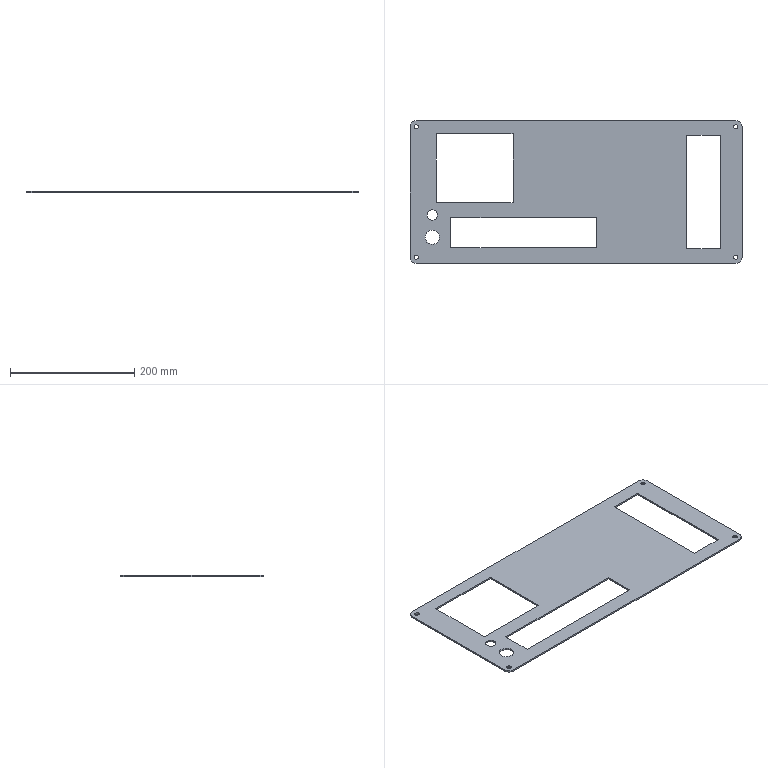Part | SolidWorks | features ICE 6, Extrusion 1, Fillet 1, LPattern 1 | 1 solid | 34 faces | box 535 x 230 x 2.5 mm | volume 217965 mm3 | plane 18 | cylinder 16 | commonest cylinder face diameters 7 x8 20 x4 16.5 x2 23 x2
STEP:
#1=CARTESIAN_POINT('',(27.75,-152.,0.));
#2=VERTEX_POINT('',#1);
#3=CARTESIAN_POINT('',(44.25,-152.,0.));
#4=VERTEX_POINT('',#3);
#5=CARTESIAN_POINT('',(36.,-152.,0.));
#6=DIRECTION('',(0.,0.,1.));
#7=DIRECTION('',(1.,0.,0.));
#8=AXIS2_PLACEMENT_3D('',#5,#6,#7);
#9=CIRCLE('',#8,8.25);
#10=EDGE_CURVE('',#2,#4,#9,.T.);
#11=ORIENTED_EDGE('',*,*,#10,.F.);
#12=CARTESIAN_POINT('',(27.75,-152.,2.5));
#13=VERTEX_POINT('',#12);
#14=CARTESIAN_POINT('',(27.75,-152.,0.));
#15=DIRECTION('',(0.,0.,1.));
#16=VECTOR('',#15,1000.);
#17=LINE('',#14,#16);
#18=EDGE_CURVE('',#2,#13,#17,.T.);
#19=ORIENTED_EDGE('',*,*,#18,.T.);
#20=CARTESIAN_POINT('',(44.25,-152.,2.5));
#21=VERTEX_POINT('',#20);
#22=CARTESIAN_POINT('',(36.,-152.,2.5));
#23=DIRECTION('',(0.,0.,1.));
#24=DIRECTION('',(1.,0.,0.));
#25=AXIS2_PLACEMENT_3D('',#22,#23,#24);
#26=CIRCLE('',#25,8.25);
#27=EDGE_CURVE('',#13,#21,#26,.T.);
#28=ORIENTED_EDGE('',*,*,#27,.T.);
#29=CARTESIAN_POINT('',(44.25,-152.,0.));
#30=DIRECTION('',(0.,0.,1.));
#31=VECTOR('',#30,1000.);
#32=LINE('',#29,#31);
#33=EDGE_CURVE('',#4,#21,#32,.T.);
#34=ORIENTED_EDGE('',*,*,#33,.F.);
#35=EDGE_LOOP('',(#11,#19,#28,#34));
#36=FACE_OUTER_BOUND('',#35,.T.);
#37=CARTESIAN_POINT('',(36.,-152.,0.));
#38=DIRECTION('',(0.,0.,1.));
#39=DIRECTION('',(1.,0.,0.));
#40=AXIS2_PLACEMENT_3D('',#37,#38,#39);
#41=CYLINDRICAL_SURFACE('',#40,8.25);
#42=ADVANCED_FACE('',(#36),#41,.F.);
#43=CARTESIAN_POINT('',(24.5,-188.,0.));
#44=VERTEX_POINT('',#43);
#45=CARTESIAN_POINT('',(47.5,-188.,0.));
#46=VERTEX_POINT('',#45);
#47=CARTESIAN_POINT('',(36.,-188.,0.));
#48=DIRECTION('',(0.,0.,1.));
#49=DIRECTION('',(1.,0.,0.));
#50=AXIS2_PLACEMENT_3D('',#47,#48,#49);
#51=CIRCLE('',#50,11.5);
#52=EDGE_CURVE('',#44,#46,#51,.T.);
#53=ORIENTED_EDGE('',*,*,#52,.F.);
#54=CARTESIAN_POINT('',(24.5,-188.,2.5));
#55=VERTEX_POINT('',#54);
#56=CARTESIAN_POINT('',(24.5,-188.,0.));
#57=DIRECTION('',(0.,0.,1.));
#58=VECTOR('',#57,1000.);
#59=LINE('',#56,#58);
#60=EDGE_CURVE('',#44,#55,#59,.T.);
#61=ORIENTED_EDGE('',*,*,#60,.T.);
#62=CARTESIAN_POINT('',(47.5,-188.,2.5));
#63=VERTEX_POINT('',#62);
#64=CARTESIAN_POINT('',(36.,-188.,2.5));
#65=DIRECTION('',(0.,0.,1.));
#66=DIRECTION('',(1.,0.,0.));
#67=AXIS2_PLACEMENT_3D('',#64,#65,#66);
#68=CIRCLE('',#67,11.5);
#69=EDGE_CURVE('',#55,#63,#68,.T.);
#70=ORIENTED_EDGE('',*,*,#69,.T.);
#71=CARTESIAN_POINT('',(47.5,-188.,0.));
#72=DIRECTION('',(0.,0.,1.));
#73=VECTOR('',#72,1000.);
#74=LINE('',#71,#73);
#75=EDGE_CURVE('',#46,#63,#74,.T.);
#76=ORIENTED_EDGE('',*,*,#75,.F.);
#77=EDGE_LOOP('',(#53,#61,#70,#76));
#78=FACE_OUTER_BOUND('',#77,.T.);
#79=CARTESIAN_POINT('',(36.,-188.,0.));
#80=DIRECTION('',(0.,0.,1.));
#81=DIRECTION('',(1.,0.,0.));
#82=AXIS2_PLACEMENT_3D('',#79,#80,#81);
#83=CYLINDRICAL_SURFACE('',#82,11.5);
#84=ADVANCED_FACE('',(#78),#83,.F.);
#85=CARTESIAN_POINT('',(521.5,-220.,0.));
#86=VERTEX_POINT('',#85);
#87=CARTESIAN_POINT('',(528.5,-220.,0.));
#88=VERTEX_POINT('',#87);
#89=CARTESIAN_POINT('',(525.,-220.,0.));
#90=DIRECTION('',(0.,0.,1.));
#91=DIRECTION('',(1.,0.,0.));
#92=AXIS2_PLACEMENT_3D('',#89,#90,#91);
#93=CIRCLE('',#92,3.5);
#94=EDGE_CURVE('',#86,#88,#93,.T.);
#95=ORIENTED_EDGE('',*,*,#94,.F.);
#96=CARTESIAN_POINT('',(521.5,-220.,2.5));
#97=VERTEX_POINT('',#96);
#98=CARTESIAN_POINT('',(521.5,-220.,0.));
#99=DIRECTION('',(0.,0.,1.));
#100=VECTOR('',#99,1000.);
#101=LINE('',#98,#100);
#102=EDGE_CURVE('',#86,#97,#101,.T.);
#103=ORIENTED_EDGE('',*,*,#102,.T.);
#104=CARTESIAN_POINT('',(528.5,-220.,2.5));
#105=VERTEX_POINT('',#104);
#106=CARTESIAN_POINT('',(525.,-220.,2.5));
#107=DIRECTION('',(0.,0.,1.));
#108=DIRECTION('',(1.,0.,0.));
#109=AXIS2_PLACEMENT_3D('',#106,#107,#108);
#110=CIRCLE('',#109,3.5);
#111=EDGE_CURVE('',#97,#105,#110,.T.);
#112=ORIENTED_EDGE('',*,*,#111,.T.);
#113=CARTESIAN_POINT('',(528.5,-220.,0.));
#114=DIRECTION('',(0.,0.,1.));
#115=VECTOR('',#114,1000.);
#116=LINE('',#113,#115);
#117=EDGE_CURVE('',#88,#105,#116,.T.);
#118=ORIENTED_EDGE('',*,*,#117,.F.);
#119=EDGE_LOOP('',(#95,#103,#112,#118));
#120=FACE_OUTER_BOUND('',#119,.T.);
#121=CARTESIAN_POINT('',(525.,-220.,0.));
#122=DIRECTION('',(0.,0.,1.));
#123=DIRECTION('',(1.,0.,0.));
#124=AXIS2_PLACEMENT_3D('',#121,#122,#123);
#125=CYLINDRICAL_SURFACE('',#124,3.5);
#126=ADVANCED_FACE('',(#120),#125,.F.);
#127=CARTESIAN_POINT('',(521.5,-10.,0.));
#128=VERTEX_POINT('',#127);
#129=CARTESIAN_POINT('',(528.5,-10.,0.));
#130=VERTEX_POINT('',#129);
#131=CARTESIAN_POINT('',(525.,-10.,0.));
#132=DIRECTION('',(0.,0.,1.));
#133=DIRECTION('',(1.,0.,0.));
#134=AXIS2_PLACEMENT_3D('',#131,#132,#133);
#135=CIRCLE('',#134,3.5);
#136=EDGE_CURVE('',#128,#130,#135,.T.);
#137=ORIENTED_EDGE('',*,*,#136,.F.);
#138=CARTESIAN_POINT('',(521.5,-10.,2.5));
#139=VERTEX_POINT('',#138);
#140=CARTESIAN_POINT('',(521.5,-10.,0.));
#141=DIRECTION('',(0.,0.,1.));
#142=VECTOR('',#141,1000.);
#143=LINE('',#140,#142);
#144=EDGE_CURVE('',#128,#139,#143,.T.);
#145=ORIENTED_EDGE('',*,*,#144,.T.);
#146=CARTESIAN_POINT('',(528.5,-10.,2.5));
#147=VERTEX_POINT('',#146);
#148=CARTESIAN_POINT('',(525.,-10.,2.5));
#149=DIRECTION('',(0.,0.,1.));
#150=DIRECTION('',(1.,0.,0.));
#151=AXIS2_PLACEMENT_3D('',#148,#149,#150);
#152=CIRCLE('',#151,3.5);
#153=EDGE_CURVE('',#139,#147,#152,.T.);
#154=ORIENTED_EDGE('',*,*,#153,.T.);
#155=CARTESIAN_POINT('',(528.5,-10.,0.));
#156=DIRECTION('',(0.,0.,1.));
#157=VECTOR('',#156,1000.);
#158=LINE('',#155,#157);
#159=EDGE_CURVE('',#130,#147,#158,.T.);
#160=ORIENTED_EDGE('',*,*,#159,.F.);
#161=EDGE_LOOP('',(#137,#145,#154,#160));
#162=FACE_OUTER_BOUND('',#161,.T.);
#163=CARTESIAN_POINT('',(525.,-10.,0.));
#164=DIRECTION('',(0.,0.,1.));
#165=DIRECTION('',(1.,0.,0.));
#166=AXIS2_PLACEMENT_3D('',#163,#164,#165);
#167=CYLINDRICAL_SURFACE('',#166,3.5);
#168=ADVANCED_FACE('',(#162),#167,.F.);
#169=CARTESIAN_POINT('',(6.5,-220.,0.));
#170=VERTEX_POINT('',#169);
#171=CARTESIAN_POINT('',(13.5,-220.,0.));
#172=VERTEX_POINT('',#171);
#173=CARTESIAN_POINT('',(10.,-220.,0.));
#174=DIRECTION('',(0.,0.,1.));
#175=DIRECTION('',(1.,0.,0.));
#176=AXIS2_PLACEMENT_3D('',#173,#174,#175);
#177=CIRCLE('',#176,3.5);
#178=EDGE_CURVE('',#170,#172,#177,.T.);
#179=ORIENTED_EDGE('',*,*,#178,.F.);
#180=CARTESIAN_POINT('',(6.5,-220.,2.5));
#181=VERTEX_POINT('',#180);
#182=CARTESIAN_POINT('',(6.5,-220.,0.));
#183=DIRECTION('',(0.,0.,1.));
#184=VECTOR('',#183,1000.);
#185=LINE('',#182,#184);
#186=EDGE_CURVE('',#170,#181,#185,.T.);
#187=ORIENTED_EDGE('',*,*,#186,.T.);
#188=CARTESIAN_POINT('',(13.5,-220.,2.5));
#189=VERTEX_POINT('',#188);
#190=CARTESIAN_POINT('',(10.,-220.,2.5));
#191=DIRECTION('',(0.,0.,1.));
#192=DIRECTION('',(1.,0.,0.));
#193=AXIS2_PLACEMENT_3D('',#190,#191,#192);
#194=CIRCLE('',#193,3.5);
#195=EDGE_CURVE('',#181,#189,#194,.T.);
#196=ORIENTED_EDGE('',*,*,#195,.T.);
#197=CARTESIAN_POINT('',(13.5,-220.,0.));
#198=DIRECTION('',(0.,0.,1.));
#199=VECTOR('',#198,1000.);
#200=LINE('',#197,#199);
#201=EDGE_CURVE('',#172,#189,#200,.T.);
#202=ORIENTED_EDGE('',*,*,#201,.F.);
#203=EDGE_LOOP('',(#179,#187,#196,#202));
#204=FACE_OUTER_BOUND('',#203,.T.);
#205=CARTESIAN_POINT('',(10.,-220.,0.));
#206=DIRECTION('',(0.,0.,1.));
#207=DIRECTION('',(1.,0.,0.));
#208=AXIS2_PLACEMENT_3D('',#205,#206,#207);
#209=CYLINDRICAL_SURFACE('',#208,3.5);
#210=ADVANCED_FACE('',(#204),#209,.F.);
#211=CARTESIAN_POINT('',(6.5,-10.,0.));
#212=VERTEX_POINT('',#211);
#213=CARTESIAN_POINT('',(13.5,-10.,0.));
#214=VERTEX_POINT('',#213);
#215=CARTESIAN_POINT('',(10.,-10.,0.));
#216=DIRECTION('',(0.,0.,1.));
#217=DIRECTION('',(1.,0.,0.));
#218=AXIS2_PLACEMENT_3D('',#215,#216,#217);
#219=CIRCLE('',#218,3.5);
#220=EDGE_CURVE('',#212,#214,#219,.T.);
#221=ORIENTED_EDGE('',*,*,#220,.F.);
#222=CARTESIAN_POINT('',(6.5,-10.,2.5));
#223=VERTEX_POINT('',#222);
#224=CARTESIAN_POINT('',(6.5,-10.,0.));
#225=DIRECTION('',(0.,0.,1.));
#226=VECTOR('',#225,1000.);
#227=LINE('',#224,#226);
#228=EDGE_CURVE('',#212,#223,#227,.T.);
#229=ORIENTED_EDGE('',*,*,#228,.T.);
#230=CARTESIAN_POINT('',(13.5,-10.,2.5));
#231=VERTEX_POINT('',#230);
#232=CARTESIAN_POINT('',(10.,-10.,2.5));
#233=DIRECTION('',(0.,0.,1.));
#234=DIRECTION('',(1.,0.,0.));
#235=AXIS2_PLACEMENT_3D('',#232,#233,#234);
#236=CIRCLE('',#235,3.5);
#237=EDGE_CURVE('',#223,#231,#236,.T.);
#238=ORIENTED_EDGE('',*,*,#237,.T.);
#239=CARTESIAN_POINT('',(13.5,-10.,0.));
#240=DIRECTION('',(0.,0.,1.));
#241=VECTOR('',#240,1000.);
#242=LINE('',#239,#241);
#243=EDGE_CURVE('',#214,#231,#242,.T.);
#244=ORIENTED_EDGE('',*,*,#243,.F.);
#245=EDGE_LOOP('',(#221,#229,#238,#244));
#246=FACE_OUTER_BOUND('',#245,.T.);
#247=CARTESIAN_POINT('',(10.,-10.,0.));
#248=DIRECTION('',(0.,0.,1.));
#249=DIRECTION('',(1.,0.,0.));
#250=AXIS2_PLACEMENT_3D('',#247,#248,#249);
#251=CYLINDRICAL_SURFACE('',#250,3.5);
#252=ADVANCED_FACE('',(#246),#251,.F.);
#253=CARTESIAN_POINT('',(0.,-10.,0.));
#254=VERTEX_POINT('',#253);
#255=CARTESIAN_POINT('',(0.,-220.,0.));
#256=VERTEX_POINT('',#255);
#257=CARTESIAN_POINT('',(0.,0.,0.));
#258=DIRECTION('',(0.,-1.,0.));
#259=VECTOR('',#258,1000.);
#260=LINE('',#257,#259);
#261=EDGE_CURVE('',#254,#256,#260,.T.);
#262=ORIENTED_EDGE('',*,*,#261,.T.);
#263=CARTESIAN_POINT('',(0.,-220.,2.5));
#264=VERTEX_POINT('',#263);
#265=CARTESIAN_POINT('',(0.,-220.,2.5));
#266=DIRECTION('',(0.,0.,1.));
#267=VECTOR('',#266,1000.);
#268=LINE('',#265,#267);
#269=EDGE_CURVE('',#256,#264,#268,.T.);
#270=ORIENTED_EDGE('',*,*,#269,.T.);
#271=CARTESIAN_POINT('',(0.,-10.,2.5));
#272=VERTEX_POINT('',#271);
#273=CARTESIAN_POINT('',(0.,0.,2.5));
#274=DIRECTION('',(0.,-1.,0.));
#275=VECTOR('',#274,1000.);
#276=LINE('',#273,#275);
#277=EDGE_CURVE('',#272,#264,#276,.T.);
#278=ORIENTED_EDGE('',*,*,#277,.F.);
#279=CARTESIAN_POINT('',(0.,-10.,2.5));
#280=DIRECTION('',(0.,0.,-1.));
#281=VECTOR('',#280,1000.);
#282=LINE('',#279,#281);
#283=EDGE_CURVE('',#272,#254,#282,.T.);
#284=ORIENTED_EDGE('',*,*,#283,.T.);
#285=EDGE_LOOP('',(#262,#270,#278,#284));
#286=FACE_OUTER_BOUND('',#285,.T.);
#287=CARTESIAN_POINT('',(0.,0.,2.5));
#288=DIRECTION('',(1.,0.,0.));
#289=DIRECTION('',(0.,1.,0.));
#290=AXIS2_PLACEMENT_3D('',#287,#288,#289);
#291=PLANE('',#290);
#292=ADVANCED_FACE('',(#286),#291,.F.);
#293=CARTESIAN_POINT('',(10.,-230.,2.5));
#294=VERTEX_POINT('',#293);
#295=CARTESIAN_POINT('',(525.,-230.,2.5));
#296=VERTEX_POINT('',#295);
#297=CARTESIAN_POINT('',(0.,-230.,2.5));
#298=DIRECTION('',(1.,0.,0.));
#299=VECTOR('',#298,1000.);
#300=LINE('',#297,#299);
#301=EDGE_CURVE('',#294,#296,#300,.T.);
#302=ORIENTED_EDGE('',*,*,#301,.F.);
#303=CARTESIAN_POINT('',(10.,-230.,0.));
#304=VERTEX_POINT('',#303);
#305=CARTESIAN_POINT('',(10.,-230.,2.5));
#306=DIRECTION('',(0.,0.,-1.));
#307=VECTOR('',#306,1000.);
#308=LINE('',#305,#307);
#309=EDGE_CURVE('',#294,#304,#308,.T.);
#310=ORIENTED_EDGE('',*,*,#309,.T.);
#311=CARTESIAN_POINT('',(525.,-230.,0.));
#312=VERTEX_POINT('',#311);
#313=CARTESIAN_POINT('',(0.,-230.,0.));
#314=DIRECTION('',(1.,0.,0.));
#315=VECTOR('',#314,1000.);
#316=LINE('',#313,#315);
#317=EDGE_CURVE('',#304,#312,#316,.T.);
#318=ORIENTED_EDGE('',*,*,#317,.T.);
#319=CARTESIAN_POINT('',(525.,-230.,2.5));
#320=DIRECTION('',(0.,0.,1.));
#321=VECTOR('',#320,1000.);
#322=LINE('',#319,#321);
#323=EDGE_CURVE('',#312,#296,#322,.T.);
#324=ORIENTED_EDGE('',*,*,#323,.T.);
#325=EDGE_LOOP('',(#302,#310,#318,#324));
#326=FACE_OUTER_BOUND('',#325,.T.);
#327=CARTESIAN_POINT('',(0.,-230.,2.5));
#328=DIRECTION('',(0.,1.,0.));
#329=DIRECTION('',(0.,0.,1.));
#330=AXIS2_PLACEMENT_3D('',#327,#328,#329);
#331=PLANE('',#330);
#332=ADVANCED_FACE('',(#326),#331,.F.);
#333=CARTESIAN_POINT('',(535.,-220.,2.5));
#334=VERTEX_POINT('',#333);
#335=CARTESIAN_POINT('',(535.,-10.,2.5));
#336=VERTEX_POINT('',#335);
#337=CARTESIAN_POINT('',(535.,0.,2.5));
#338=DIRECTION('',(0.,1.,0.));
#339=VECTOR('',#338,1000.);
#340=LINE('',#337,#339);
#341=EDGE_CURVE('',#334,#336,#340,.T.);
#342=ORIENTED_EDGE('',*,*,#341,.F.);
#343=CARTESIAN_POINT('',(535.,-220.,0.));
#344=VERTEX_POINT('',#343);
#345=CARTESIAN_POINT('',(535.,-220.,2.5));
#346=DIRECTION('',(0.,0.,-1.));
#347=VECTOR('',#346,1000.);
#348=LINE('',#345,#347);
#349=EDGE_CURVE('',#334,#344,#348,.T.);
#350=ORIENTED_EDGE('',*,*,#349,.T.);
#351=CARTESIAN_POINT('',(535.,-10.,0.));
#352=VERTEX_POINT('',#351);
#353=CARTESIAN_POINT('',(535.,0.,0.));
#354=DIRECTION('',(0.,1.,0.));
#355=VECTOR('',#354,1000.);
#356=LINE('',#353,#355);
#357=EDGE_CURVE('',#344,#352,#356,.T.);
#358=ORIENTED_EDGE('',*,*,#357,.T.);
#359=CARTESIAN_POINT('',(535.,-10.,2.5));
#360=DIRECTION('',(0.,0.,1.));
#361=VECTOR('',#360,1000.);
#362=LINE('',#359,#361);
#363=EDGE_CURVE('',#352,#336,#362,.T.);
#364=ORIENTED_EDGE('',*,*,#363,.T.);
#365=EDGE_LOOP('',(#342,#350,#358,#364));
#366=FACE_OUTER_BOUND('',#365,.T.);
#367=CARTESIAN_POINT('',(535.,0.,2.5));
#368=DIRECTION('',(-1.,0.,0.));
#369=DIRECTION('',(0.,0.,1.));
#370=AXIS2_PLACEMENT_3D('',#367,#368,#369);
#371=PLANE('',#370);
#372=ADVANCED_FACE('',(#366),#371,.F.);
#373=CARTESIAN_POINT('',(525.,0.,2.5));
#374=VERTEX_POINT('',#373);
#375=CARTESIAN_POINT('',(10.,0.,2.5));
#376=VERTEX_POINT('',#375);
#377=CARTESIAN_POINT('',(0.,0.,2.5));
#378=DIRECTION('',(-1.,0.,0.));
#379=VECTOR('',#378,1000.);
#380=LINE('',#377,#379);
#381=EDGE_CURVE('',#374,#376,#380,.T.);
#382=ORIENTED_EDGE('',*,*,#381,.F.);
#383=CARTESIAN_POINT('',(525.,0.,0.));
#384=VERTEX_POINT('',#383);
#385=CARTESIAN_POINT('',(525.,0.,2.5));
#386=DIRECTION('',(0.,0.,-1.));
#387=VECTOR('',#386,1000.);
#388=LINE('',#385,#387);
#389=EDGE_CURVE('',#374,#384,#388,.T.);
#390=ORIENTED_EDGE('',*,*,#389,.T.);
#391=CARTESIAN_POINT('',(10.,0.,0.));
#392=VERTEX_POINT('',#391);
#393=CARTESIAN_POINT('',(0.,0.,0.));
#394=DIRECTION('',(-1.,0.,0.));
#395=VECTOR('',#394,1000.);
#396=LINE('',#393,#395);
#397=EDGE_CURVE('',#384,#392,#396,.T.);
#398=ORIENTED_EDGE('',*,*,#397,.T.);
#399=CARTESIAN_POINT('',(10.,0.,2.5));
#400=DIRECTION('',(0.,0.,1.));
#401=VECTOR('',#400,1000.);
#402=LINE('',#399,#401);
#403=EDGE_CURVE('',#392,#376,#402,.T.);
#404=ORIENTED_EDGE('',*,*,#403,.T.);
#405=EDGE_LOOP('',(#382,#390,#398,#404));
#406=FACE_OUTER_BOUND('',#405,.T.);
#407=CARTESIAN_POINT('',(0.,0.,2.5));
#408=DIRECTION('',(0.,-1.,0.));
#409=DIRECTION('',(0.,0.,-1.));
#410=AXIS2_PLACEMENT_3D('',#407,#408,#409);
#411=PLANE('',#410);
#412=ADVANCED_FACE('',(#406),#411,.F.);
#413=CARTESIAN_POINT('',(446.,-23.5,2.5));
#414=VERTEX_POINT('',#413);
#415=CARTESIAN_POINT('',(446.,-206.5,2.5));
#416=VERTEX_POINT('',#415);
#417=CARTESIAN_POINT('',(446.,-23.5,2.5));
#418=DIRECTION('',(0.,-1.,0.));
#419=VECTOR('',#418,1000.);
#420=LINE('',#417,#419);
#421=EDGE_CURVE('',#414,#416,#420,.T.);
#422=ORIENTED_EDGE('',*,*,#421,.F.);
#423=CARTESIAN_POINT('',(500.,-23.5,2.5));
#424=VERTEX_POINT('',#423);
#425=CARTESIAN_POINT('',(446.,-23.5,2.5));
#426=DIRECTION('',(-1.,0.,0.));
#427=VECTOR('',#426,1000.);
#428=LINE('',#425,#427);
#429=EDGE_CURVE('',#424,#414,#428,.T.);
#430=ORIENTED_EDGE('',*,*,#429,.F.);
#431=CARTESIAN_POINT('',(500.,-206.5,2.5));
#432=VERTEX_POINT('',#431);
#433=CARTESIAN_POINT('',(500.,-23.5,2.5));
#434=DIRECTION('',(0.,1.,0.));
#435=VECTOR('',#434,1000.);
#436=LINE('',#433,#435);
#437=EDGE_CURVE('',#432,#424,#436,.T.);
#438=ORIENTED_EDGE('',*,*,#437,.F.);
#439=CARTESIAN_POINT('',(446.,-206.5,2.5));
#440=DIRECTION('',(1.,0.,0.));
#441=VECTOR('',#440,1000.);
#442=LINE('',#439,#441);
#443=EDGE_CURVE('',#416,#432,#442,.T.);
#444=ORIENTED_EDGE('',*,*,#443,.F.);
#445=EDGE_LOOP('',(#422,#430,#438,#444));
#446=FACE_BOUND('',#445,.T.);
#447=CARTESIAN_POINT('',(36.,-152.,2.5));
#448=DIRECTION('',(0.,0.,1.));
#449=DIRECTION('',(1.,0.,0.));
#450=AXIS2_PLACEMENT_3D('',#447,#448,#449);
#451=CIRCLE('',#450,8.25);
#452=EDGE_CURVE('',#21,#13,#451,.T.);
#453=ORIENTED_EDGE('',*,*,#452,.F.);
#454=ORIENTED_EDGE('',*,*,#27,.F.);
#455=EDGE_LOOP('',(#453,#454));
#456=FACE_BOUND('',#455,.T.);
#457=CARTESIAN_POINT('',(36.,-188.,2.5));
#458=DIRECTION('',(0.,0.,1.));
#459=DIRECTION('',(1.,0.,0.));
#460=AXIS2_PLACEMENT_3D('',#457,#458,#459);
#461=CIRCLE('',#460,11.5);
#462=EDGE_CURVE('',#63,#55,#461,.T.);
#463=ORIENTED_EDGE('',*,*,#462,.F.);
#464=ORIENTED_EDGE('',*,*,#69,.F.);
#465=EDGE_LOOP('',(#463,#464));
#466=FACE_BOUND('',#465,.T.);
#467=CARTESIAN_POINT('',(66.,-156.5,2.5));
#468=VERTEX_POINT('',#467);
#469=CARTESIAN_POINT('',(66.,-205.,2.5));
#470=VERTEX_POINT('',#469);
#471=CARTESIAN_POINT('',(66.,-156.5,2.5));
#472=DIRECTION('',(0.,-1.,0.));
#473=VECTOR('',#472,1000.);
#474=LINE('',#471,#473);
#475=EDGE_CURVE('',#468,#470,#474,.T.);
#476=ORIENTED_EDGE('',*,*,#475,.F.);
#477=CARTESIAN_POINT('',(300.,-156.5,2.5));
#478=VERTEX_POINT('',#477);
#479=CARTESIAN_POINT('',(66.,-156.5,2.5));
#480=DIRECTION('',(-1.,0.,0.));
#481=VECTOR('',#480,1000.);
#482=LINE('',#479,#481);
#483=EDGE_CURVE('',#478,#468,#482,.T.);
#484=ORIENTED_EDGE('',*,*,#483,.F.);
#485=CARTESIAN_POINT('',(300.,-205.,2.5));
#486=VERTEX_POINT('',#485);
#487=CARTESIAN_POINT('',(300.,-156.5,2.5));
#488=DIRECTION('',(0.,1.,0.));
#489=VECTOR('',#488,1000.);
#490=LINE('',#487,#489);
#491=EDGE_CURVE('',#486,#478,#490,.T.);
#492=ORIENTED_EDGE('',*,*,#491,.F.);
#493=CARTESIAN_POINT('',(66.,-205.,2.5));
#494=DIRECTION('',(1.,0.,0.));
#495=VECTOR('',#494,1000.);
#496=LINE('',#493,#495);
#497=EDGE_CURVE('',#470,#486,#496,.T.);
#498=ORIENTED_EDGE('',*,*,#497,.F.);
#499=EDGE_LOOP('',(#476,#484,#492,#498));
#500=FACE_BOUND('',#499,.T.);
#501=CARTESIAN_POINT('',(42.,-21.,2.5));
#502=VERTEX_POINT('',#501);
#503=CARTESIAN_POINT('',(42.,-132.,2.5));
#504=VERTEX_POINT('',#503);
#505=CARTESIAN_POINT('',(42.,-21.,2.5));
#506=DIRECTION('',(0.,-1.,0.));
#507=VECTOR('',#506,1000.);
#508=LINE('',#505,#507);
#509=EDGE_CURVE('',#502,#504,#508,.T.);
#510=ORIENTED_EDGE('',*,*,#509,.F.);
#511=CARTESIAN_POINT('',(166.,-21.,2.5));
#512=VERTEX_POINT('',#511);
#513=CARTESIAN_POINT('',(42.,-21.,2.5));
#514=DIRECTION('',(-1.,0.,0.));
#515=VECTOR('',#514,1000.);
#516=LINE('',#513,#515);
#517=EDGE_CURVE('',#512,#502,#516,.T.);
#518=ORIENTED_EDGE('',*,*,#517,.F.);
#519=CARTESIAN_POINT('',(166.,-132.,2.5));
#520=VERTEX_POINT('',#519);
#521=CARTESIAN_POINT('',(166.,-21.,2.5));
#522=DIRECTION('',(0.,1.,0.));
#523=VECTOR('',#522,1000.);
#524=LINE('',#521,#523);
#525=EDGE_CURVE('',#520,#512,#524,.T.);
#526=ORIENTED_EDGE('',*,*,#525,.F.);
#527=CARTESIAN_POINT('',(42.,-132.,2.5));
#528=DIRECTION('',(1.,0.,0.));
#529=VECTOR('',#528,1000.);
#530=LINE('',#527,#529);
#531=EDGE_CURVE('',#504,#520,#530,.T.);
#532=ORIENTED_EDGE('',*,*,#531,.F.);
#533=EDGE_LOOP('',(#510,#518,#526,#532));
#534=FACE_BOUND('',#533,.T.);
#535=CARTESIAN_POINT('',(525.,-220.,2.5));
#536=DIRECTION('',(0.,0.,1.));
#537=DIRECTION('',(1.,0.,0.));
#538=AXIS2_PLACEMENT_3D('',#535,#536,#537);
#539=CIRCLE('',#538,3.5);
#540=EDGE_CURVE('',#105,#97,#539,.T.);
#541=ORIENTED_EDGE('',*,*,#540,.F.);
#542=ORIENTED_EDGE('',*,*,#111,.F.);
#543=EDGE_LOOP('',(#541,#542));
#544=FACE_BOUND('',#543,.T.);
#545=CARTESIAN_POINT('',(525.,-10.,2.5));
#546=DIRECTION('',(0.,0.,1.));
#547=DIRECTION('',(1.,0.,0.));
#548=AXIS2_PLACEMENT_3D('',#545,#546,#547);
#549=CIRCLE('',#548,3.5);
#550=EDGE_CURVE('',#147,#139,#549,.T.);
#551=ORIENTED_EDGE('',*,*,#550,.F.);
#552=ORIENTED_EDGE('',*,*,#153,.F.);
#553=EDGE_LOOP('',(#551,#552));
#554=FACE_BOUND('',#553,.T.);
#555=CARTESIAN_POINT('',(10.,-220.,2.5));
#556=DIRECTION('',(0.,0.,1.));
#557=DIRECTION('',(1.,0.,0.));
#558=AXIS2_PLACEMENT_3D('',#555,#556,#557);
#559=CIRCLE('',#558,3.5);
#560=EDGE_CURVE('',#189,#181,#559,.T.);
#561=ORIENTED_EDGE('',*,*,#560,.F.);
#562=ORIENTED_EDGE('',*,*,#195,.F.);
#563=EDGE_LOOP('',(#561,#562));
#564=FACE_BOUND('',#563,.T.);
#565=CARTESIAN_POINT('',(10.,-10.,2.5));
#566=DIRECTION('',(0.,0.,1.));
#567=DIRECTION('',(1.,0.,0.));
#568=AXIS2_PLACEMENT_3D('',#565,#566,#567);
#569=CIRCLE('',#568,3.5);
#570=EDGE_CURVE('',#231,#223,#569,.T.);
#571=ORIENTED_EDGE('',*,*,#570,.F.);
#572=ORIENTED_EDGE('',*,*,#237,.F.);
#573=EDGE_LOOP('',(#571,#572));
#574=FACE_BOUND('',#573,.T.);
#575=ORIENTED_EDGE('',*,*,#277,.T.);
#576=CARTESIAN_POINT('',(10.,-220.,2.5));
#577=DIRECTION('',(0.,0.,1.));
#578=DIRECTION('',(1.,0.,0.));
#579=AXIS2_PLACEMENT_3D('',#576,#577,#578);
#580=CIRCLE('',#579,10.);
#581=EDGE_CURVE('',#264,#294,#580,.T.);
#582=ORIENTED_EDGE('',*,*,#581,.T.);
#583=ORIENTED_EDGE('',*,*,#301,.T.);
#584=CARTESIAN_POINT('',(525.,-220.,2.5));
#585=DIRECTION('',(0.,0.,1.));
#586=DIRECTION('',(1.,0.,0.));
#587=AXIS2_PLACEMENT_3D('',#584,#585,#586);
#588=CIRCLE('',#587,10.);
#589=EDGE_CURVE('',#296,#334,#588,.T.);
#590=ORIENTED_EDGE('',*,*,#589,.T.);
#591=ORIENTED_EDGE('',*,*,#341,.T.);
#592=CARTESIAN_POINT('',(525.,-10.,2.5));
#593=DIRECTION('',(0.,0.,1.));
#594=DIRECTION('',(1.,0.,0.));
#595=AXIS2_PLACEMENT_3D('',#592,#593,#594);
#596=CIRCLE('',#595,10.);
#597=EDGE_CURVE('',#336,#374,#596,.T.);
#598=ORIENTED_EDGE('',*,*,#597,.T.);
#599=ORIENTED_EDGE('',*,*,#381,.T.);
#600=CARTESIAN_POINT('',(10.,-10.,2.5));
#601=DIRECTION('',(0.,0.,1.));
#602=DIRECTION('',(1.,0.,0.));
#603=AXIS2_PLACEMENT_3D('',#600,#601,#602);
#604=CIRCLE('',#603,10.);
#605=EDGE_CURVE('',#376,#272,#604,.T.);
#606=ORIENTED_EDGE('',*,*,#605,.T.);
#607=EDGE_LOOP('',(#575,#582,#583,#590,#591,#598,#599,#606));
#608=FACE_OUTER_BOUND('',#607,.T.);
#609=CARTESIAN_POINT('',(0.,0.,2.5));
#610=DIRECTION('',(0.,0.,1.));
#611=DIRECTION('',(1.,0.,0.));
#612=AXIS2_PLACEMENT_3D('',#609,#610,#611);
#613=PLANE('',#612);
#614=ADVANCED_FACE('',(#446,#456,#466,#500,#534,#544,#554,#564,#574,#608),#613,.T.);
#615=CARTESIAN_POINT('',(500.,-23.5,0.));
#616=VERTEX_POINT('',#615);
#617=CARTESIAN_POINT('',(446.,-23.5,0.));
#618=VERTEX_POINT('',#617);
#619=CARTESIAN_POINT('',(446.,-23.5,0.));
#620=DIRECTION('',(-1.,0.,0.));
#621=VECTOR('',#620,1000.);
#622=LINE('',#619,#621);
#623=EDGE_CURVE('',#616,#618,#622,.T.);
#624=ORIENTED_EDGE('',*,*,#623,.T.);
#625=CARTESIAN_POINT('',(446.,-206.5,0.));
#626=VERTEX_POINT('',#625);
#627=CARTESIAN_POINT('',(446.,-23.5,0.));
#628=DIRECTION('',(0.,-1.,0.));
#629=VECTOR('',#628,1000.);
#630=LINE('',#627,#629);
#631=EDGE_CURVE('',#618,#626,#630,.T.);
#632=ORIENTED_EDGE('',*,*,#631,.T.);
#633=CARTESIAN_POINT('',(500.,-206.5,0.));
#634=VERTEX_POINT('',#633);
#635=CARTESIAN_POINT('',(446.,-206.5,0.));
#636=DIRECTION('',(1.,0.,0.));
#637=VECTOR('',#636,1000.);
#638=LINE('',#635,#637);
#639=EDGE_CURVE('',#626,#634,#638,.T.);
#640=ORIENTED_EDGE('',*,*,#639,.T.);
#641=CARTESIAN_POINT('',(500.,-23.5,0.));
#642=DIRECTION('',(0.,1.,0.));
#643=VECTOR('',#642,1000.);
#644=LINE('',#641,#643);
#645=EDGE_CURVE('',#634,#616,#644,.T.);
#646=ORIENTED_EDGE('',*,*,#645,.T.);
#647=EDGE_LOOP('',(#624,#632,#640,#646));
#648=FACE_BOUND('',#647,.T.);
#649=CARTESIAN_POINT('',(36.,-152.,0.));
#650=DIRECTION('',(0.,0.,1.));
#651=DIRECTION('',(1.,0.,0.));
#652=AXIS2_PLACEMENT_3D('',#649,#650,#651);
#653=CIRCLE('',#652,8.25);
#654=EDGE_CURVE('',#4,#2,#653,.T.);
#655=ORIENTED_EDGE('',*,*,#654,.T.);
#656=ORIENTED_EDGE('',*,*,#10,.T.);
#657=EDGE_LOOP('',(#655,#656));
#658=FACE_BOUND('',#657,.T.);
#659=CARTESIAN_POINT('',(36.,-188.,0.));
#660=DIRECTION('',(0.,0.,1.));
#661=DIRECTION('',(1.,0.,0.));
#662=AXIS2_PLACEMENT_3D('',#659,#660,#661);
#663=CIRCLE('',#662,11.5);
#664=EDGE_CURVE('',#46,#44,#663,.T.);
#665=ORIENTED_EDGE('',*,*,#664,.T.);
#666=ORIENTED_EDGE('',*,*,#52,.T.);
#667=EDGE_LOOP('',(#665,#666));
#668=FACE_BOUND('',#667,.T.);
#669=CARTESIAN_POINT('',(300.,-156.5,0.));
#670=VERTEX_POINT('',#669);
#671=CARTESIAN_POINT('',(66.,-156.5,0.));
#672=VERTEX_POINT('',#671);
#673=CARTESIAN_POINT('',(66.,-156.5,0.));
#674=DIRECTION('',(-1.,0.,0.));
#675=VECTOR('',#674,1000.);
#676=LINE('',#673,#675);
#677=EDGE_CURVE('',#670,#672,#676,.T.);
#678=ORIENTED_EDGE('',*,*,#677,.T.);
#679=CARTESIAN_POINT('',(66.,-205.,0.));
#680=VERTEX_POINT('',#679);
#681=CARTESIAN_POINT('',(66.,-156.5,0.));
#682=DIRECTION('',(0.,-1.,0.));
#683=VECTOR('',#682,1000.);
#684=LINE('',#681,#683);
#685=EDGE_CURVE('',#672,#680,#684,.T.);
#686=ORIENTED_EDGE('',*,*,#685,.T.);
#687=CARTESIAN_POINT('',(300.,-205.,0.));
#688=VERTEX_POINT('',#687);
#689=CARTESIAN_POINT('',(66.,-205.,0.));
#690=DIRECTION('',(1.,0.,0.));
#691=VECTOR('',#690,1000.);
#692=LINE('',#689,#691);
#693=EDGE_CURVE('',#680,#688,#692,.T.);
#694=ORIENTED_EDGE('',*,*,#693,.T.);
#695=CARTESIAN_POINT('',(300.,-156.5,0.));
#696=DIRECTION('',(0.,1.,0.));
#697=VECTOR('',#696,1000.);
#698=LINE('',#695,#697);
#699=EDGE_CURVE('',#688,#670,#698,.T.);
#700=ORIENTED_EDGE('',*,*,#699,.T.);
#701=EDGE_LOOP('',(#678,#686,#694,#700));
#702=FACE_BOUND('',#701,.T.);
#703=CARTESIAN_POINT('',(166.,-21.,0.));
#704=VERTEX_POINT('',#703);
#705=CARTESIAN_POINT('',(42.,-21.,0.));
#706=VERTEX_POINT('',#705);
#707=CARTESIAN_POINT('',(42.,-21.,0.));
#708=DIRECTION('',(-1.,0.,0.));
#709=VECTOR('',#708,1000.);
#710=LINE('',#707,#709);
#711=EDGE_CURVE('',#704,#706,#710,.T.);
#712=ORIENTED_EDGE('',*,*,#711,.T.);
#713=CARTESIAN_POINT('',(42.,-132.,0.));
#714=VERTEX_POINT('',#713);
#715=CARTESIAN_POINT('',(42.,-21.,0.));
#716=DIRECTION('',(0.,-1.,0.));
#717=VECTOR('',#716,1000.);
#718=LINE('',#715,#717);
#719=EDGE_CURVE('',#706,#714,#718,.T.);
#720=ORIENTED_EDGE('',*,*,#719,.T.);
#721=CARTESIAN_POINT('',(166.,-132.,0.));
#722=VERTEX_POINT('',#721);
#723=CARTESIAN_POINT('',(42.,-132.,0.));
#724=DIRECTION('',(1.,0.,0.));
#725=VECTOR('',#724,1000.);
#726=LINE('',#723,#725);
#727=EDGE_CURVE('',#714,#722,#726,.T.);
#728=ORIENTED_EDGE('',*,*,#727,.T.);
#729=CARTESIAN_POINT('',(166.,-21.,0.));
#730=DIRECTION('',(0.,1.,0.));
#731=VECTOR('',#730,1000.);
#732=LINE('',#729,#731);
#733=EDGE_CURVE('',#722,#704,#732,.T.);
#734=ORIENTED_EDGE('',*,*,#733,.T.);
#735=EDGE_LOOP('',(#712,#720,#728,#734));
#736=FACE_BOUND('',#735,.T.);
#737=CARTESIAN_POINT('',(525.,-220.,0.));
#738=DIRECTION('',(0.,0.,1.));
#739=DIRECTION('',(1.,0.,0.));
#740=AXIS2_PLACEMENT_3D('',#737,#738,#739);
#741=CIRCLE('',#740,3.5);
#742=EDGE_CURVE('',#88,#86,#741,.T.);
#743=ORIENTED_EDGE('',*,*,#742,.T.);
#744=ORIENTED_EDGE('',*,*,#94,.T.);
#745=EDGE_LOOP('',(#743,#744));
#746=FACE_BOUND('',#745,.T.);
#747=CARTESIAN_POINT('',(525.,-10.,0.));
#748=DIRECTION('',(0.,0.,1.));
#749=DIRECTION('',(1.,0.,0.));
#750=AXIS2_PLACEMENT_3D('',#747,#748,#749);
#751=CIRCLE('',#750,3.5);
#752=EDGE_CURVE('',#130,#128,#751,.T.);
#753=ORIENTED_EDGE('',*,*,#752,.T.);
#754=ORIENTED_EDGE('',*,*,#136,.T.);
#755=EDGE_LOOP('',(#753,#754));
#756=FACE_BOUND('',#755,.T.);
#757=CARTESIAN_POINT('',(10.,-220.,0.));
#758=DIRECTION('',(0.,0.,1.));
#759=DIRECTION('',(1.,0.,0.));
#760=AXIS2_PLACEMENT_3D('',#757,#758,#759);
#761=CIRCLE('',#760,3.5);
#762=EDGE_CURVE('',#172,#170,#761,.T.);
#763=ORIENTED_EDGE('',*,*,#762,.T.);
#764=ORIENTED_EDGE('',*,*,#178,.T.);
#765=EDGE_LOOP('',(#763,#764));
#766=FACE_BOUND('',#765,.T.);
#767=CARTESIAN_POINT('',(10.,-10.,0.));
#768=DIRECTION('',(0.,0.,1.));
#769=DIRECTION('',(1.,0.,0.));
#770=AXIS2_PLACEMENT_3D('',#767,#768,#769);
#771=CIRCLE('',#770,3.5);
#772=EDGE_CURVE('',#214,#212,#771,.T.);
#773=ORIENTED_EDGE('',*,*,#772,.T.);
#774=ORIENTED_EDGE('',*,*,#220,.T.);
#775=EDGE_LOOP('',(#773,#774));
#776=FACE_BOUND('',#775,.T.);
#777=ORIENTED_EDGE('',*,*,#317,.F.);
#778=CARTESIAN_POINT('',(10.,-220.,0.));
#779=DIRECTION('',(0.,0.,-1.));
#780=DIRECTION('',(1.,0.,0.));
#781=AXIS2_PLACEMENT_3D('',#778,#779,#780);
#782=CIRCLE('',#781,10.);
#783=EDGE_CURVE('',#304,#256,#782,.T.);
#784=ORIENTED_EDGE('',*,*,#783,.T.);
#785=ORIENTED_EDGE('',*,*,#261,.F.);
#786=CARTESIAN_POINT('',(10.,-10.,0.));
#787=DIRECTION('',(0.,0.,-1.));
#788=DIRECTION('',(1.,0.,0.));
#789=AXIS2_PLACEMENT_3D('',#786,#787,#788);
#790=CIRCLE('',#789,10.);
#791=EDGE_CURVE('',#254,#392,#790,.T.);
#792=ORIENTED_EDGE('',*,*,#791,.T.);
#793=ORIENTED_EDGE('',*,*,#397,.F.);
#794=CARTESIAN_POINT('',(525.,-10.,0.));
#795=DIRECTION('',(0.,0.,-1.));
#796=DIRECTION('',(1.,0.,0.));
#797=AXIS2_PLACEMENT_3D('',#794,#795,#796);
#798=CIRCLE('',#797,10.);
#799=EDGE_CURVE('',#384,#352,#798,.T.);
#800=ORIENTED_EDGE('',*,*,#799,.T.);
#801=ORIENTED_EDGE('',*,*,#357,.F.);
#802=CARTESIAN_POINT('',(525.,-220.,0.));
#803=DIRECTION('',(0.,0.,-1.));
#804=DIRECTION('',(1.,0.,0.));
#805=AXIS2_PLACEMENT_3D('',#802,#803,#804);
#806=CIRCLE('',#805,10.);
#807=EDGE_CURVE('',#344,#312,#806,.T.);
#808=ORIENTED_EDGE('',*,*,#807,.T.);
#809=EDGE_LOOP('',(#777,#784,#785,#792,#793,#800,#801,#808));
#810=FACE_OUTER_BOUND('',#809,.T.);
#811=CARTESIAN_POINT('',(0.,0.,0.));
#812=DIRECTION('',(0.,0.,1.));
#813=DIRECTION('',(1.,0.,0.));
#814=AXIS2_PLACEMENT_3D('',#811,#812,#813);
#815=PLANE('',#814);
#816=ADVANCED_FACE('',(#648,#658,#668,#702,#736,#746,#756,#766,#776,#810),#815,.F.);
#817=ORIENTED_EDGE('',*,*,#581,.F.);
#818=ORIENTED_EDGE('',*,*,#269,.F.);
#819=ORIENTED_EDGE('',*,*,#783,.F.);
#820=ORIENTED_EDGE('',*,*,#309,.F.);
#821=EDGE_LOOP('',(#817,#818,#819,#820));
#822=FACE_OUTER_BOUND('',#821,.T.);
#823=CARTESIAN_POINT('',(10.,-220.,2.5));
#824=DIRECTION('',(0.,0.,-1.));
#825=DIRECTION('',(-1.,0.,0.));
#826=AXIS2_PLACEMENT_3D('',#823,#824,#825);
#827=CYLINDRICAL_SURFACE('',#826,10.);
#828=ADVANCED_FACE('',(#822),#827,.T.);
#829=ORIENTED_EDGE('',*,*,#589,.F.);
#830=ORIENTED_EDGE('',*,*,#323,.F.);
#831=ORIENTED_EDGE('',*,*,#807,.F.);
#832=ORIENTED_EDGE('',*,*,#349,.F.);
#833=EDGE_LOOP('',(#829,#830,#831,#832));
#834=FACE_OUTER_BOUND('',#833,.T.);
#835=CARTESIAN_POINT('',(525.,-220.,2.5));
#836=DIRECTION('',(0.,0.,-1.));
#837=DIRECTION('',(-1.,0.,0.));
#838=AXIS2_PLACEMENT_3D('',#835,#836,#837);
#839=CYLINDRICAL_SURFACE('',#838,10.);
#840=ADVANCED_FACE('',(#834),#839,.T.);
#841=ORIENTED_EDGE('',*,*,#597,.F.);
#842=ORIENTED_EDGE('',*,*,#363,.F.);
#843=ORIENTED_EDGE('',*,*,#799,.F.);
#844=ORIENTED_EDGE('',*,*,#389,.F.);
#845=EDGE_LOOP('',(#841,#842,#843,#844));
#846=FACE_OUTER_BOUND('',#845,.T.);
#847=CARTESIAN_POINT('',(525.,-10.,2.5));
#848=DIRECTION('',(0.,0.,-1.));
#849=DIRECTION('',(-1.,0.,0.));
#850=AXIS2_PLACEMENT_3D('',#847,#848,#849);
#851=CYLINDRICAL_SURFACE('',#850,10.);
#852=ADVANCED_FACE('',(#846),#851,.T.);
#853=ORIENTED_EDGE('',*,*,#605,.F.);
#854=ORIENTED_EDGE('',*,*,#403,.F.);
#855=ORIENTED_EDGE('',*,*,#791,.F.);
#856=ORIENTED_EDGE('',*,*,#283,.F.);
#857=EDGE_LOOP('',(#853,#854,#855,#856));
#858=FACE_OUTER_BOUND('',#857,.T.);
#859=CARTESIAN_POINT('',(10.,-10.,2.5));
#860=DIRECTION('',(0.,0.,-1.));
#861=DIRECTION('',(-1.,0.,0.));
#862=AXIS2_PLACEMENT_3D('',#859,#860,#861);
#863=CYLINDRICAL_SURFACE('',#862,10.);
#864=ADVANCED_FACE('',(#858),#863,.T.);
#865=ORIENTED_EDGE('',*,*,#228,.F.);
#866=ORIENTED_EDGE('',*,*,#772,.F.);
#867=ORIENTED_EDGE('',*,*,#243,.T.);
#868=ORIENTED_EDGE('',*,*,#570,.T.);
#869=EDGE_LOOP('',(#865,#866,#867,#868));
#870=FACE_OUTER_BOUND('',#869,.T.);
#871=CARTESIAN_POINT('',(10.,-10.,0.));
#872=DIRECTION('',(0.,0.,1.));
#873=DIRECTION('',(1.,0.,0.));
#874=AXIS2_PLACEMENT_3D('',#871,#872,#873);
#875=CYLINDRICAL_SURFACE('',#874,3.5);
#876=ADVANCED_FACE('',(#870),#875,.F.);
#877=ORIENTED_EDGE('',*,*,#186,.F.);
#878=ORIENTED_EDGE('',*,*,#762,.F.);
#879=ORIENTED_EDGE('',*,*,#201,.T.);
#880=ORIENTED_EDGE('',*,*,#560,.T.);
#881=EDGE_LOOP('',(#877,#878,#879,#880));
#882=FACE_OUTER_BOUND('',#881,.T.);
#883=CARTESIAN_POINT('',(10.,-220.,0.));
#884=DIRECTION('',(0.,0.,1.));
#885=DIRECTION('',(1.,0.,0.));
#886=AXIS2_PLACEMENT_3D('',#883,#884,#885);
#887=CYLINDRICAL_SURFACE('',#886,3.5);
#888=ADVANCED_FACE('',(#882),#887,.F.);
#889=ORIENTED_EDGE('',*,*,#144,.F.);
#890=ORIENTED_EDGE('',*,*,#752,.F.);
#891=ORIENTED_EDGE('',*,*,#159,.T.);
#892=ORIENTED_EDGE('',*,*,#550,.T.);
#893=EDGE_LOOP('',(#889,#890,#891,#892));
#894=FACE_OUTER_BOUND('',#893,.T.);
#895=CARTESIAN_POINT('',(525.,-10.,0.));
#896=DIRECTION('',(0.,0.,1.));
#897=DIRECTION('',(1.,0.,0.));
#898=AXIS2_PLACEMENT_3D('',#895,#896,#897);
#899=CYLINDRICAL_SURFACE('',#898,3.5);
#900=ADVANCED_FACE('',(#894),#899,.F.);
#901=ORIENTED_EDGE('',*,*,#102,.F.);
#902=ORIENTED_EDGE('',*,*,#742,.F.);
#903=ORIENTED_EDGE('',*,*,#117,.T.);
#904=ORIENTED_EDGE('',*,*,#540,.T.);
#905=EDGE_LOOP('',(#901,#902,#903,#904));
#906=FACE_OUTER_BOUND('',#905,.T.);
#907=CARTESIAN_POINT('',(525.,-220.,0.));
#908=DIRECTION('',(0.,0.,1.));
#909=DIRECTION('',(1.,0.,0.));
#910=AXIS2_PLACEMENT_3D('',#907,#908,#909);
#911=CYLINDRICAL_SURFACE('',#910,3.5);
#912=ADVANCED_FACE('',(#906),#911,.F.);
#913=ORIENTED_EDGE('',*,*,#509,.T.);
#914=CARTESIAN_POINT('',(42.,-132.,0.));
#915=DIRECTION('',(0.,0.,1.));
#916=VECTOR('',#915,1000.);
#917=LINE('',#914,#916);
#918=EDGE_CURVE('',#714,#504,#917,.T.);
#919=ORIENTED_EDGE('',*,*,#918,.F.);
#920=ORIENTED_EDGE('',*,*,#719,.F.);
#921=CARTESIAN_POINT('',(42.,-21.,0.));
#922=DIRECTION('',(0.,0.,1.));
#923=VECTOR('',#922,1000.);
#924=LINE('',#921,#923);
#925=EDGE_CURVE('',#706,#502,#924,.T.);
#926=ORIENTED_EDGE('',*,*,#925,.T.);
#927=EDGE_LOOP('',(#913,#919,#920,#926));
#928=FACE_OUTER_BOUND('',#927,.T.);
#929=CARTESIAN_POINT('',(42.,-21.,0.));
#930=DIRECTION('',(-1.,0.,0.));
#931=DIRECTION('',(0.,-1.,0.));
#932=AXIS2_PLACEMENT_3D('',#929,#930,#931);
#933=PLANE('',#932);
#934=ADVANCED_FACE('',(#928),#933,.F.);
#935=ORIENTED_EDGE('',*,*,#517,.T.);
#936=ORIENTED_EDGE('',*,*,#925,.F.);
#937=ORIENTED_EDGE('',*,*,#711,.F.);
#938=CARTESIAN_POINT('',(166.,-21.,0.));
#939=DIRECTION('',(0.,0.,1.));
#940=VECTOR('',#939,1000.);
#941=LINE('',#938,#940);
#942=EDGE_CURVE('',#704,#512,#941,.T.);
#943=ORIENTED_EDGE('',*,*,#942,.T.);
#944=EDGE_LOOP('',(#935,#936,#937,#943));
#945=FACE_OUTER_BOUND('',#944,.T.);
#946=CARTESIAN_POINT('',(42.,-21.,0.));
#947=DIRECTION('',(0.,1.,0.));
#948=DIRECTION('',(0.,0.,1.));
#949=AXIS2_PLACEMENT_3D('',#946,#947,#948);
#950=PLANE('',#949);
#951=ADVANCED_FACE('',(#945),#950,.F.);
#952=ORIENTED_EDGE('',*,*,#525,.T.);
#953=ORIENTED_EDGE('',*,*,#942,.F.);
#954=ORIENTED_EDGE('',*,*,#733,.F.);
#955=CARTESIAN_POINT('',(166.,-132.,0.));
#956=DIRECTION('',(0.,0.,1.));
#957=VECTOR('',#956,1000.);
#958=LINE('',#955,#957);
#959=EDGE_CURVE('',#722,#520,#958,.T.);
#960=ORIENTED_EDGE('',*,*,#959,.T.);
#961=EDGE_LOOP('',(#952,#953,#954,#960));
#962=FACE_OUTER_BOUND('',#961,.T.);
#963=CARTESIAN_POINT('',(166.,-21.,0.));
#964=DIRECTION('',(1.,0.,0.));
#965=DIRECTION('',(0.,0.,-1.));
#966=AXIS2_PLACEMENT_3D('',#963,#964,#965);
#967=PLANE('',#966);
#968=ADVANCED_FACE('',(#962),#967,.F.);
#969=ORIENTED_EDGE('',*,*,#531,.T.);
#970=ORIENTED_EDGE('',*,*,#959,.F.);
#971=ORIENTED_EDGE('',*,*,#727,.F.);
#972=ORIENTED_EDGE('',*,*,#918,.T.);
#973=EDGE_LOOP('',(#969,#970,#971,#972));
#974=FACE_OUTER_BOUND('',#973,.T.);
#975=CARTESIAN_POINT('',(42.,-132.,0.));
#976=DIRECTION('',(0.,-1.,0.));
#977=DIRECTION('',(0.,0.,-1.));
#978=AXIS2_PLACEMENT_3D('',#975,#976,#977);
#979=PLANE('',#978);
#980=ADVANCED_FACE('',(#974),#979,.F.);
#981=ORIENTED_EDGE('',*,*,#475,.T.);
#982=CARTESIAN_POINT('',(66.,-205.,0.));
#983=DIRECTION('',(0.,0.,1.));
#984=VECTOR('',#983,1000.);
#985=LINE('',#982,#984);
#986=EDGE_CURVE('',#680,#470,#985,.T.);
#987=ORIENTED_EDGE('',*,*,#986,.F.);
#988=ORIENTED_EDGE('',*,*,#685,.F.);
#989=CARTESIAN_POINT('',(66.,-156.5,0.));
#990=DIRECTION('',(0.,0.,1.));
#991=VECTOR('',#990,1000.);
#992=LINE('',#989,#991);
#993=EDGE_CURVE('',#672,#468,#992,.T.);
#994=ORIENTED_EDGE('',*,*,#993,.T.);
#995=EDGE_LOOP('',(#981,#987,#988,#994));
#996=FACE_OUTER_BOUND('',#995,.T.);
#997=CARTESIAN_POINT('',(66.,-156.5,0.));
#998=DIRECTION('',(-1.,0.,0.));
#999=DIRECTION('',(0.,0.,1.));
#1000=AXIS2_PLACEMENT_3D('',#997,#998,#999);
#1001=PLANE('',#1000);
#1002=ADVANCED_FACE('',(#996),#1001,.F.);
#1003=ORIENTED_EDGE('',*,*,#483,.T.);
#1004=ORIENTED_EDGE('',*,*,#993,.F.);
#1005=ORIENTED_EDGE('',*,*,#677,.F.);
#1006=CARTESIAN_POINT('',(300.,-156.5,0.));
#1007=DIRECTION('',(0.,0.,1.));
#1008=VECTOR('',#1007,1000.);
#1009=LINE('',#1006,#1008);
#1010=EDGE_CURVE('',#670,#478,#1009,.T.);
#1011=ORIENTED_EDGE('',*,*,#1010,.T.);
#1012=EDGE_LOOP('',(#1003,#1004,#1005,#1011));
#1013=FACE_OUTER_BOUND('',#1012,.T.);
#1014=CARTESIAN_POINT('',(66.,-156.5,0.));
#1015=DIRECTION('',(0.,1.,0.));
#1016=DIRECTION('',(0.,0.,1.));
#1017=AXIS2_PLACEMENT_3D('',#1014,#1015,#1016);
#1018=PLANE('',#1017);
#1019=ADVANCED_FACE('',(#1013),#1018,.F.);
#1020=ORIENTED_EDGE('',*,*,#491,.T.);
#1021=ORIENTED_EDGE('',*,*,#1010,.F.);
#1022=ORIENTED_EDGE('',*,*,#699,.F.);
#1023=CARTESIAN_POINT('',(300.,-205.,0.));
#1024=DIRECTION('',(0.,0.,1.));
#1025=VECTOR('',#1024,1000.);
#1026=LINE('',#1023,#1025);
#1027=EDGE_CURVE('',#688,#486,#1026,.T.);
#1028=ORIENTED_EDGE('',*,*,#1027,.T.);
#1029=EDGE_LOOP('',(#1020,#1021,#1022,#1028));
#1030=FACE_OUTER_BOUND('',#1029,.T.);
#1031=CARTESIAN_POINT('',(300.,-156.5,0.));
#1032=DIRECTION('',(1.,0.,0.));
#1033=DIRECTION('',(0.,0.,-1.));
#1034=AXIS2_PLACEMENT_3D('',#1031,#1032,#1033);
#1035=PLANE('',#1034);
#1036=ADVANCED_FACE('',(#1030),#1035,.F.);
#1037=ORIENTED_EDGE('',*,*,#497,.T.);
#1038=ORIENTED_EDGE('',*,*,#1027,.F.);
#1039=ORIENTED_EDGE('',*,*,#693,.F.);
#1040=ORIENTED_EDGE('',*,*,#986,.T.);
#1041=EDGE_LOOP('',(#1037,#1038,#1039,#1040));
#1042=FACE_OUTER_BOUND('',#1041,.T.);
#1043=CARTESIAN_POINT('',(66.,-205.,0.));
#1044=DIRECTION('',(0.,-1.,0.));
#1045=DIRECTION('',(0.,0.,-1.));
#1046=AXIS2_PLACEMENT_3D('',#1043,#1044,#1045);
#1047=PLANE('',#1046);
#1048=ADVANCED_FACE('',(#1042),#1047,.F.);
#1049=ORIENTED_EDGE('',*,*,#60,.F.);
#1050=ORIENTED_EDGE('',*,*,#664,.F.);
#1051=ORIENTED_EDGE('',*,*,#75,.T.);
#1052=ORIENTED_EDGE('',*,*,#462,.T.);
#1053=EDGE_LOOP('',(#1049,#1050,#1051,#1052));
#1054=FACE_OUTER_BOUND('',#1053,.T.);
#1055=CARTESIAN_POINT('',(36.,-188.,0.));
#1056=DIRECTION('',(0.,0.,1.));
#1057=DIRECTION('',(1.,0.,0.));
#1058=AXIS2_PLACEMENT_3D('',#1055,#1056,#1057);
#1059=CYLINDRICAL_SURFACE('',#1058,11.5);
#1060=ADVANCED_FACE('',(#1054),#1059,.F.);
#1061=ORIENTED_EDGE('',*,*,#18,.F.);
#1062=ORIENTED_EDGE('',*,*,#654,.F.);
#1063=ORIENTED_EDGE('',*,*,#33,.T.);
#1064=ORIENTED_EDGE('',*,*,#452,.T.);
#1065=EDGE_LOOP('',(#1061,#1062,#1063,#1064));
#1066=FACE_OUTER_BOUND('',#1065,.T.);
#1067=CARTESIAN_POINT('',(36.,-152.,0.));
#1068=DIRECTION('',(0.,0.,1.));
#1069=DIRECTION('',(1.,0.,0.));
#1070=AXIS2_PLACEMENT_3D('',#1067,#1068,#1069);
#1071=CYLINDRICAL_SURFACE('',#1070,8.25);
#1072=ADVANCED_FACE('',(#1066),#1071,.F.);
#1073=ORIENTED_EDGE('',*,*,#421,.T.);
#1074=CARTESIAN_POINT('',(446.,-206.5,0.));
#1075=DIRECTION('',(0.,0.,1.));
#1076=VECTOR('',#1075,1000.);
#1077=LINE('',#1074,#1076);
#1078=EDGE_CURVE('',#626,#416,#1077,.T.);
#1079=ORIENTED_EDGE('',*,*,#1078,.F.);
#1080=ORIENTED_EDGE('',*,*,#631,.F.);
#1081=CARTESIAN_POINT('',(446.,-23.5,0.));
#1082=DIRECTION('',(0.,0.,1.));
#1083=VECTOR('',#1082,1000.);
#1084=LINE('',#1081,#1083);
#1085=EDGE_CURVE('',#618,#414,#1084,.T.);
#1086=ORIENTED_EDGE('',*,*,#1085,.T.);
#1087=EDGE_LOOP('',(#1073,#1079,#1080,#1086));
#1088=FACE_OUTER_BOUND('',#1087,.T.);
#1089=CARTESIAN_POINT('',(446.,-23.5,0.));
#1090=DIRECTION('',(-1.,0.,0.));
#1091=DIRECTION('',(0.,-1.,0.));
#1092=AXIS2_PLACEMENT_3D('',#1089,#1090,#1091);
#1093=PLANE('',#1092);
#1094=ADVANCED_FACE('',(#1088),#1093,.F.);
#1095=ORIENTED_EDGE('',*,*,#429,.T.);
#1096=ORIENTED_EDGE('',*,*,#1085,.F.);
#1097=ORIENTED_EDGE('',*,*,#623,.F.);
#1098=CARTESIAN_POINT('',(500.,-23.5,0.));
#1099=DIRECTION('',(0.,0.,1.));
#1100=VECTOR('',#1099,1000.);
#1101=LINE('',#1098,#1100);
#1102=EDGE_CURVE('',#616,#424,#1101,.T.);
#1103=ORIENTED_EDGE('',*,*,#1102,.T.);
#1104=EDGE_LOOP('',(#1095,#1096,#1097,#1103));
#1105=FACE_OUTER_BOUND('',#1104,.T.);
#1106=CARTESIAN_POINT('',(446.,-23.5,0.));
#1107=DIRECTION('',(0.,1.,0.));
#1108=DIRECTION('',(0.,0.,1.));
#1109=AXIS2_PLACEMENT_3D('',#1106,#1107,#1108);
#1110=PLANE('',#1109);
#1111=ADVANCED_FACE('',(#1105),#1110,.F.);
#1112=ORIENTED_EDGE('',*,*,#437,.T.);
#1113=ORIENTED_EDGE('',*,*,#1102,.F.);
#1114=ORIENTED_EDGE('',*,*,#645,.F.);
#1115=CARTESIAN_POINT('',(500.,-206.5,0.));
#1116=DIRECTION('',(0.,0.,1.));
#1117=VECTOR('',#1116,1000.);
#1118=LINE('',#1115,#1117);
#1119=EDGE_CURVE('',#634,#432,#1118,.T.);
#1120=ORIENTED_EDGE('',*,*,#1119,.T.);
#1121=EDGE_LOOP('',(#1112,#1113,#1114,#1120));
#1122=FACE_OUTER_BOUND('',#1121,.T.);
#1123=CARTESIAN_POINT('',(500.,-23.5,0.));
#1124=DIRECTION('',(1.,0.,0.));
#1125=DIRECTION('',(0.,0.,-1.));
#1126=AXIS2_PLACEMENT_3D('',#1123,#1124,#1125);
#1127=PLANE('',#1126);
#1128=ADVANCED_FACE('',(#1122),#1127,.F.);
#1129=ORIENTED_EDGE('',*,*,#443,.T.);
#1130=ORIENTED_EDGE('',*,*,#1119,.F.);
#1131=ORIENTED_EDGE('',*,*,#639,.F.);
#1132=ORIENTED_EDGE('',*,*,#1078,.T.);
#1133=EDGE_LOOP('',(#1129,#1130,#1131,#1132));
#1134=FACE_OUTER_BOUND('',#1133,.T.);
#1135=CARTESIAN_POINT('',(446.,-206.5,0.));
#1136=DIRECTION('',(0.,-1.,0.));
#1137=DIRECTION('',(0.,0.,-1.));
#1138=AXIS2_PLACEMENT_3D('',#1135,#1136,#1137);
#1139=PLANE('',#1138);
#1140=ADVANCED_FACE('',(#1134),#1139,.F.);
#1141=CLOSED_SHELL('',(#42,#84,#126,#168,#210,#252,#292,#332,#372,#412,#614,#816,#828,#840,#852,#864,#876,#888,#900,#912,#934,#951,#968,#980,#1002,#1019,#1036,#1048,#1060,#1072,#1094,#1111,#1128,#1140));
#1142=MANIFOLD_SOLID_BREP('',#1141);
#1143=CARTESIAN_POINT('',(0.,0.,0.));
#1144=DIRECTION('',(0.,0.,1.));
#1145=DIRECTION('',(1.,0.,0.));
#1146=AXIS2_PLACEMENT_3D('',#1143,#1144,#1145);
#1147=(LENGTH_UNIT()NAMED_UNIT(*)SI_UNIT(.MILLI.,.METRE.));
#1148=UNCERTAINTY_MEASURE_WITH_UNIT(LENGTH_MEASURE(0.00001),#1147,'','');
#1149=(NAMED_UNIT(*)PLANE_ANGLE_UNIT()SI_UNIT($,.RADIAN.));
#1150=(NAMED_UNIT(*)SI_UNIT($,.STERADIAN.)SOLID_ANGLE_UNIT());
#1151=(GEOMETRIC_REPRESENTATION_CONTEXT(3)GLOBAL_UNCERTAINTY_ASSIGNED_CONTEXT((#1148))GLOBAL_UNIT_ASSIGNED_CONTEXT((#1147,#1149,#1150))REPRESENTATION_CONTEXT('',''));
#1152=ADVANCED_BREP_SHAPE_REPRESENTATION('',(#1142,#1146),#1151);